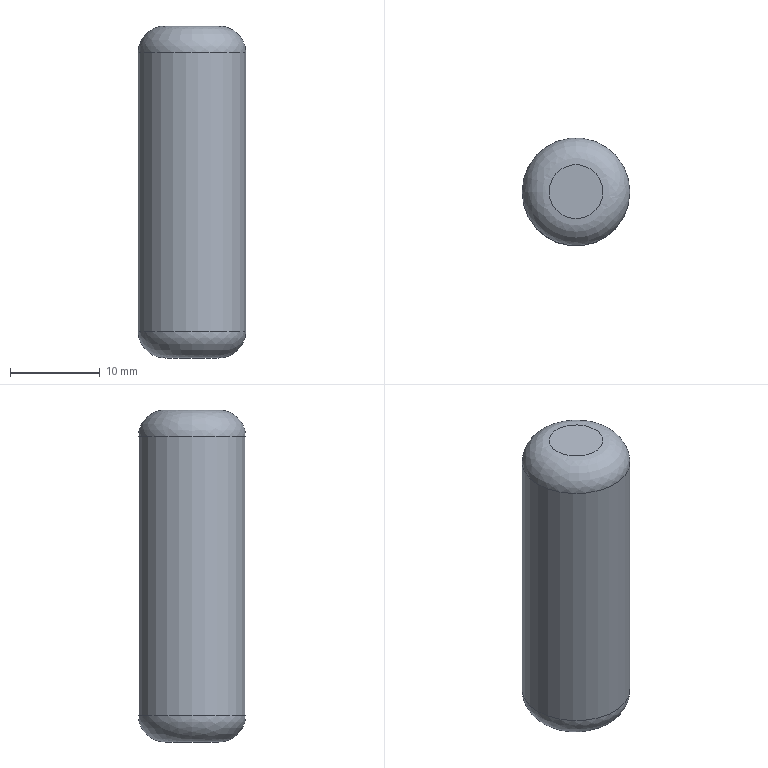Part | STEP file | Tube feed_id1566_x_t | 1 solid | 5 faces | box 12 x 12 x 37 mm | volume 4054 mm3 | plane 2 | spline 2 | cylinder 1 | commonest cylinder face diameters 12 x1
STEP:
#1=CARTESIAN_POINT('',(0.,0.,0.));
#2=DIRECTION('',(0.,0.,1.));
#3=DIRECTION('',(1.,0.,0.));
#4=AXIS2_PLACEMENT_3D('',#1,#2,#3);
#5=CARTESIAN_POINT('',(-15.,508.136,-235.));
#6=VERTEX_POINT('',#5);
#7=CARTESIAN_POINT('',(-9.,508.136,-235.));
#8=DIRECTION('',(0.,0.,1.));
#9=DIRECTION('',(-1.,0.,0.));
#10=AXIS2_PLACEMENT_3D('',#7,#8,#9);
#11=CIRCLE('',#10,6.);
#12=CARTESIAN_POINT('',(-9.,508.136,-201.));
#13=DIRECTION('',(0.,0.,-1.));
#14=DIRECTION('',(-1.,0.,0.));
#15=AXIS2_PLACEMENT_3D('',#12,#13,#14);
#16=CYLINDRICAL_SURFACE('',#15,6.);
#17=CARTESIAN_POINT('',(6.283,34.));
#18=DIRECTION('',(-1.,0.));
#19=VECTOR('',#18,1.);
#20=LINE('',#17,#19);
#21=(GEOMETRIC_REPRESENTATION_CONTEXT(2)PARAMETRIC_REPRESENTATION_CONTEXT()REPRESENTATION_CONTEXT('',''));
#22=DEFINITIONAL_REPRESENTATION('',(#20),#21);
#23=PCURVE('',#16,#22);
#24=CARTESIAN_POINT('',(-12.,508.136,-238.));
#25=CARTESIAN_POINT('',(-12.,514.136,-238.));
#26=CARTESIAN_POINT('',(-6.,514.136,-238.));
#27=CARTESIAN_POINT('',(-6.,508.136,-238.));
#28=CARTESIAN_POINT('',(-6.,502.136,-238.));
#29=CARTESIAN_POINT('',(-12.,502.136,-238.));
#30=CARTESIAN_POINT('',(-12.,508.136,-238.));
#31=CARTESIAN_POINT('',(-13.757,508.136,-238.));
#32=CARTESIAN_POINT('',(-13.757,517.65,-238.));
#33=CARTESIAN_POINT('',(-4.243,517.65,-238.));
#34=CARTESIAN_POINT('',(-4.243,508.136,-238.));
#35=CARTESIAN_POINT('',(-4.243,498.621,-238.));
#36=CARTESIAN_POINT('',(-13.757,498.621,-238.));
#37=CARTESIAN_POINT('',(-13.757,508.136,-238.));
#38=CARTESIAN_POINT('',(-15.,508.136,-236.757));
#39=CARTESIAN_POINT('',(-15.,520.136,-236.757));
#40=CARTESIAN_POINT('',(-3.,520.136,-236.757));
#41=CARTESIAN_POINT('',(-3.,508.136,-236.757));
#42=CARTESIAN_POINT('',(-3.,496.136,-236.757));
#43=CARTESIAN_POINT('',(-15.,496.136,-236.757));
#44=CARTESIAN_POINT('',(-15.,508.136,-236.757));
#45=CARTESIAN_POINT('',(-15.,508.136,-235.));
#46=CARTESIAN_POINT('',(-15.,520.136,-235.));
#47=CARTESIAN_POINT('',(-3.,520.136,-235.));
#48=CARTESIAN_POINT('',(-3.,508.136,-235.));
#49=CARTESIAN_POINT('',(-3.,496.136,-235.));
#50=CARTESIAN_POINT('',(-15.,496.136,-235.));
#51=CARTESIAN_POINT('',(-15.,508.136,-235.));
#52=(BOUNDED_SURFACE()B_SPLINE_SURFACE(3,3,((#24,#25,#26,#27,#28,#29,#30),(#31,#32,#33,#34,#35,#36,#37),(#38,#39,#40,#41,#42,#43,#44),(#45,#46,#47,#48,#49,#50,#51)),.UNSPECIFIED.,.F.,.T.,.F.)B_SPLINE_SURFACE_WITH_KNOTS((4,4),(1,3,3,3,1),(0.,1.),(-0.5,0.,0.5,1.,1.5),.UNSPECIFIED.)GEOMETRIC_REPRESENTATION_ITEM()RATIONAL_B_SPLINE_SURFACE(((1.,0.3333,0.3333,1.,0.3333,0.3333,1.),(0.8047,0.2682,0.2682,0.8047,0.2682,0.2682,0.8047),(0.8047,0.2682,0.2682,0.8047,0.2682,0.2682,0.8047),(1.,0.3333,0.3333,1.,0.3333,0.3333,1.)))REPRESENTATION_ITEM('')SURFACE());
#53=CARTESIAN_POINT('',(1.,1.));
#54=CARTESIAN_POINT('',(1.,0.9765));
#55=CARTESIAN_POINT('',(1.,0.9351));
#56=CARTESIAN_POINT('',(1.,0.8854));
#57=CARTESIAN_POINT('',(1.,0.8425));
#58=CARTESIAN_POINT('',(1.,0.804));
#59=CARTESIAN_POINT('',(1.,0.7678));
#60=CARTESIAN_POINT('',(1.,0.7322));
#61=CARTESIAN_POINT('',(1.,0.696));
#62=CARTESIAN_POINT('',(1.,0.6575));
#63=CARTESIAN_POINT('',(1.,0.6144));
#64=CARTESIAN_POINT('',(1.,0.5657));
#65=CARTESIAN_POINT('',(1.,0.5));
#66=CARTESIAN_POINT('',(1.,0.4343));
#67=CARTESIAN_POINT('',(1.,0.3856));
#68=CARTESIAN_POINT('',(1.,0.3425));
#69=CARTESIAN_POINT('',(1.,0.304));
#70=CARTESIAN_POINT('',(1.,0.2678));
#71=CARTESIAN_POINT('',(1.,0.2322));
#72=CARTESIAN_POINT('',(1.,0.196));
#73=CARTESIAN_POINT('',(1.,0.1575));
#74=CARTESIAN_POINT('',(1.,0.1146));
#75=CARTESIAN_POINT('',(1.,0.06491));
#76=CARTESIAN_POINT('',(1.,0.02352));
#77=CARTESIAN_POINT('',(1.,0.));
#78=B_SPLINE_CURVE_WITH_KNOTS('',3,(#53,#54,#55,#56,#57,#58,#59,#60,#61,#62,#63,#64,#65,#66,#67,#68,#69,#70,#71,#72,#73,#74,#75,#76,#77),.UNSPECIFIED.,.F.,.F.,(4,1,1,1,1,1,1,1,1,1,1,1,1,1,1,1,1,1,1,1,1,1,4),(0.,0.2856,0.5712,0.8568,1.142,1.428,1.714,1.999,2.285,2.57,2.856,3.142,3.427,3.713,3.998,4.284,4.57,4.855,5.141,5.426,5.712,5.998,6.283),.QUASI_UNIFORM_KNOTS.);
#79=(GEOMETRIC_REPRESENTATION_CONTEXT(2)PARAMETRIC_REPRESENTATION_CONTEXT()REPRESENTATION_CONTEXT('',''));
#80=DEFINITIONAL_REPRESENTATION('',(#78),#79);
#81=PCURVE('',#52,#80);
#82=SURFACE_CURVE('',#11,(#23,#81),.PCURVE_S1.);
#83=EDGE_CURVE('',#6,#6,#82,.T.);
#84=ORIENTED_EDGE('',*,*,#83,.T.);
#85=CARTESIAN_POINT('',(-15.,508.136,-204.));
#86=VERTEX_POINT('',#85);
#87=CARTESIAN_POINT('',(-15.,508.136,-204.));
#88=CARTESIAN_POINT('',(-15.,508.136,-235.));
#89=B_SPLINE_CURVE_WITH_KNOTS('',1,(#87,#88),.UNSPECIFIED.,.F.,.F.,(2,2),(3.,34.),.PIECEWISE_BEZIER_KNOTS.);
#90=CARTESIAN_POINT('',(0.,0.));
#91=DIRECTION('',(0.,1.));
#92=VECTOR('',#91,1.);
#93=LINE('',#90,#92);
#94=(GEOMETRIC_REPRESENTATION_CONTEXT(2)PARAMETRIC_REPRESENTATION_CONTEXT()REPRESENTATION_CONTEXT('',''));
#95=DEFINITIONAL_REPRESENTATION('',(#93),#94);
#96=PCURVE('',#16,#95);
#97=CARTESIAN_POINT('',(6.283,0.));
#98=DIRECTION('',(0.,1.));
#99=VECTOR('',#98,1.);
#100=LINE('',#97,#99);
#101=(GEOMETRIC_REPRESENTATION_CONTEXT(2)PARAMETRIC_REPRESENTATION_CONTEXT()REPRESENTATION_CONTEXT('',''));
#102=DEFINITIONAL_REPRESENTATION('',(#100),#101);
#103=PCURVE('',#16,#102);
#104=SEAM_CURVE('',#89,(#96,#103),.PCURVE_S1.);
#105=EDGE_CURVE('',#86,#6,#104,.T.);
#106=ORIENTED_EDGE('',*,*,#105,.F.);
#107=CARTESIAN_POINT('',(-9.,508.136,-204.));
#108=DIRECTION('',(0.,0.,-1.));
#109=DIRECTION('',(-1.,0.,0.));
#110=AXIS2_PLACEMENT_3D('',#107,#108,#109);
#111=CIRCLE('',#110,6.);
#112=CARTESIAN_POINT('',(0.,3.));
#113=DIRECTION('',(1.,0.));
#114=VECTOR('',#113,1.);
#115=LINE('',#112,#114);
#116=(GEOMETRIC_REPRESENTATION_CONTEXT(2)PARAMETRIC_REPRESENTATION_CONTEXT()REPRESENTATION_CONTEXT('',''));
#117=DEFINITIONAL_REPRESENTATION('',(#115),#116);
#118=PCURVE('',#16,#117);
#119=CARTESIAN_POINT('',(-15.,508.136,-204.));
#120=CARTESIAN_POINT('',(-15.,520.136,-204.));
#121=CARTESIAN_POINT('',(-3.,520.136,-204.));
#122=CARTESIAN_POINT('',(-3.,508.136,-204.));
#123=CARTESIAN_POINT('',(-3.,496.136,-204.));
#124=CARTESIAN_POINT('',(-15.,496.136,-204.));
#125=CARTESIAN_POINT('',(-15.,508.136,-204.));
#126=CARTESIAN_POINT('',(-15.,508.136,-202.243));
#127=CARTESIAN_POINT('',(-15.,520.136,-202.243));
#128=CARTESIAN_POINT('',(-3.,520.136,-202.243));
#129=CARTESIAN_POINT('',(-3.,508.136,-202.243));
#130=CARTESIAN_POINT('',(-3.,496.136,-202.243));
#131=CARTESIAN_POINT('',(-15.,496.136,-202.243));
#132=CARTESIAN_POINT('',(-15.,508.136,-202.243));
#133=CARTESIAN_POINT('',(-13.757,508.136,-201.));
#134=CARTESIAN_POINT('',(-13.757,517.65,-201.));
#135=CARTESIAN_POINT('',(-4.243,517.65,-201.));
#136=CARTESIAN_POINT('',(-4.243,508.136,-201.));
#137=CARTESIAN_POINT('',(-4.243,498.621,-201.));
#138=CARTESIAN_POINT('',(-13.757,498.621,-201.));
#139=CARTESIAN_POINT('',(-13.757,508.136,-201.));
#140=CARTESIAN_POINT('',(-12.,508.136,-201.));
#141=CARTESIAN_POINT('',(-12.,514.136,-201.));
#142=CARTESIAN_POINT('',(-6.,514.136,-201.));
#143=CARTESIAN_POINT('',(-6.,508.136,-201.));
#144=CARTESIAN_POINT('',(-6.,502.136,-201.));
#145=CARTESIAN_POINT('',(-12.,502.136,-201.));
#146=CARTESIAN_POINT('',(-12.,508.136,-201.));
#147=(BOUNDED_SURFACE()B_SPLINE_SURFACE(3,3,((#119,#120,#121,#122,#123,#124,#125),(#126,#127,#128,#129,#130,#131,#132),(#133,#134,#135,#136,#137,#138,#139),(#140,#141,#142,#143,#144,#145,#146)),.UNSPECIFIED.,.F.,.T.,.F.)B_SPLINE_SURFACE_WITH_KNOTS((4,4),(1,3,3,3,1),(0.,1.),(-0.5,0.,0.5,1.,1.5),.UNSPECIFIED.)GEOMETRIC_REPRESENTATION_ITEM()RATIONAL_B_SPLINE_SURFACE(((1.,0.3333,0.3333,1.,0.3333,0.3333,1.),(0.8047,0.2682,0.2682,0.8047,0.2682,0.2682,0.8047),(0.8047,0.2682,0.2682,0.8047,0.2682,0.2682,0.8047),(1.,0.3333,0.3333,1.,0.3333,0.3333,1.)))REPRESENTATION_ITEM('')SURFACE());
#148=CARTESIAN_POINT('',(0.,0.));
#149=CARTESIAN_POINT('',(0.,0.02352));
#150=CARTESIAN_POINT('',(0.,0.06491));
#151=CARTESIAN_POINT('',(0.,0.1146));
#152=CARTESIAN_POINT('',(0.,0.1575));
#153=CARTESIAN_POINT('',(0.,0.196));
#154=CARTESIAN_POINT('',(0.,0.2322));
#155=CARTESIAN_POINT('',(0.,0.2678));
#156=CARTESIAN_POINT('',(0.,0.304));
#157=CARTESIAN_POINT('',(0.,0.3425));
#158=CARTESIAN_POINT('',(0.,0.3856));
#159=CARTESIAN_POINT('',(0.,0.4343));
#160=CARTESIAN_POINT('',(0.,0.5));
#161=CARTESIAN_POINT('',(0.,0.5657));
#162=CARTESIAN_POINT('',(0.,0.6144));
#163=CARTESIAN_POINT('',(0.,0.6575));
#164=CARTESIAN_POINT('',(0.,0.696));
#165=CARTESIAN_POINT('',(0.,0.7322));
#166=CARTESIAN_POINT('',(0.,0.7678));
#167=CARTESIAN_POINT('',(0.,0.804));
#168=CARTESIAN_POINT('',(0.,0.8425));
#169=CARTESIAN_POINT('',(0.,0.8854));
#170=CARTESIAN_POINT('',(0.,0.9351));
#171=CARTESIAN_POINT('',(0.,0.9765));
#172=CARTESIAN_POINT('',(0.,1.));
#173=B_SPLINE_CURVE_WITH_KNOTS('',3,(#148,#149,#150,#151,#152,#153,#154,#155,#156,#157,#158,#159,#160,#161,#162,#163,#164,#165,#166,#167,#168,#169,#170,#171,#172),.UNSPECIFIED.,.F.,.F.,(4,1,1,1,1,1,1,1,1,1,1,1,1,1,1,1,1,1,1,1,1,1,4),(0.,0.2856,0.5712,0.8568,1.142,1.428,1.714,1.999,2.285,2.57,2.856,3.142,3.427,3.713,3.998,4.284,4.57,4.855,5.141,5.426,5.712,5.998,6.283),.QUASI_UNIFORM_KNOTS.);
#174=(GEOMETRIC_REPRESENTATION_CONTEXT(2)PARAMETRIC_REPRESENTATION_CONTEXT()REPRESENTATION_CONTEXT('',''));
#175=DEFINITIONAL_REPRESENTATION('',(#173),#174);
#176=PCURVE('',#147,#175);
#177=SURFACE_CURVE('',#111,(#118,#176),.PCURVE_S1.);
#178=EDGE_CURVE('',#86,#86,#177,.T.);
#179=ORIENTED_EDGE('',*,*,#178,.T.);
#180=ORIENTED_EDGE('',*,*,#105,.T.);
#181=EDGE_LOOP('',(#84,#106,#179,#180));
#182=FACE_BOUND('',#181,.T.);
#183=ADVANCED_FACE('',(#182),#16,.T.);
#184=CARTESIAN_POINT('',(-12.,508.136,-201.));
#185=VERTEX_POINT('',#184);
#186=CARTESIAN_POINT('',(-9.,508.136,-201.));
#187=DIRECTION('',(0.,0.,1.));
#188=DIRECTION('',(-1.,0.,0.));
#189=AXIS2_PLACEMENT_3D('',#186,#187,#188);
#190=CIRCLE('',#189,3.);
#191=CARTESIAN_POINT('',(-9.,508.136,-201.));
#192=DIRECTION('',(0.,0.,-1.));
#193=DIRECTION('',(-1.,0.,0.));
#194=AXIS2_PLACEMENT_3D('',#191,#192,#193);
#195=PLANE('',#194);
#196=CARTESIAN_POINT('',(3.,0.));
#197=CARTESIAN_POINT('',(3.,-5.196));
#198=CARTESIAN_POINT('',(-1.5,-2.598));
#199=CARTESIAN_POINT('',(-6.,0.));
#200=CARTESIAN_POINT('',(-1.5,2.598));
#201=CARTESIAN_POINT('',(3.,5.196));
#202=CARTESIAN_POINT('',(3.,0.));
#203=(BOUNDED_CURVE()B_SPLINE_CURVE(2,(#196,#197,#198,#199,#200,#201,#202),.UNSPECIFIED.,.T.,.F.)B_SPLINE_CURVE_WITH_KNOTS((1,2,2,2,2,1),(-2.094,0.,2.094,4.189,6.283,8.378),.UNSPECIFIED.)CURVE()GEOMETRIC_REPRESENTATION_ITEM()RATIONAL_B_SPLINE_CURVE((1.,0.5,1.,0.5,1.,0.5,1.))REPRESENTATION_ITEM(''));
#204=(GEOMETRIC_REPRESENTATION_CONTEXT(2)PARAMETRIC_REPRESENTATION_CONTEXT()REPRESENTATION_CONTEXT('',''));
#205=DEFINITIONAL_REPRESENTATION('',(#203),#204);
#206=PCURVE('',#195,#205);
#207=CARTESIAN_POINT('',(1.,1.));
#208=CARTESIAN_POINT('',(1.,0.9765));
#209=CARTESIAN_POINT('',(1.,0.9351));
#210=CARTESIAN_POINT('',(1.,0.8854));
#211=CARTESIAN_POINT('',(1.,0.8425));
#212=CARTESIAN_POINT('',(1.,0.804));
#213=CARTESIAN_POINT('',(1.,0.7678));
#214=CARTESIAN_POINT('',(1.,0.7322));
#215=CARTESIAN_POINT('',(1.,0.696));
#216=CARTESIAN_POINT('',(1.,0.6575));
#217=CARTESIAN_POINT('',(1.,0.6144));
#218=CARTESIAN_POINT('',(1.,0.5657));
#219=CARTESIAN_POINT('',(1.,0.5));
#220=CARTESIAN_POINT('',(1.,0.4343));
#221=CARTESIAN_POINT('',(1.,0.3856));
#222=CARTESIAN_POINT('',(1.,0.3425));
#223=CARTESIAN_POINT('',(1.,0.304));
#224=CARTESIAN_POINT('',(1.,0.2678));
#225=CARTESIAN_POINT('',(1.,0.2322));
#226=CARTESIAN_POINT('',(1.,0.196));
#227=CARTESIAN_POINT('',(1.,0.1575));
#228=CARTESIAN_POINT('',(1.,0.1146));
#229=CARTESIAN_POINT('',(1.,0.06491));
#230=CARTESIAN_POINT('',(1.,0.02352));
#231=CARTESIAN_POINT('',(1.,0.));
#232=B_SPLINE_CURVE_WITH_KNOTS('',3,(#207,#208,#209,#210,#211,#212,#213,#214,#215,#216,#217,#218,#219,#220,#221,#222,#223,#224,#225,#226,#227,#228,#229,#230,#231),.UNSPECIFIED.,.F.,.F.,(4,1,1,1,1,1,1,1,1,1,1,1,1,1,1,1,1,1,1,1,1,1,4),(0.,0.2856,0.5712,0.8568,1.142,1.428,1.714,1.999,2.285,2.57,2.856,3.142,3.427,3.713,3.998,4.284,4.57,4.855,5.141,5.426,5.712,5.998,6.283),.QUASI_UNIFORM_KNOTS.);
#233=(GEOMETRIC_REPRESENTATION_CONTEXT(2)PARAMETRIC_REPRESENTATION_CONTEXT()REPRESENTATION_CONTEXT('',''));
#234=DEFINITIONAL_REPRESENTATION('',(#232),#233);
#235=PCURVE('',#147,#234);
#236=SURFACE_CURVE('',#190,(#206,#235),.PCURVE_S1.);
#237=EDGE_CURVE('',#185,#185,#236,.T.);
#238=ORIENTED_EDGE('',*,*,#237,.T.);
#239=EDGE_LOOP('',(#238));
#240=FACE_BOUND('',#239,.T.);
#241=ADVANCED_FACE('',(#240),#195,.F.);
#242=CARTESIAN_POINT('',(-12.,508.136,-238.));
#243=VERTEX_POINT('',#242);
#244=CARTESIAN_POINT('',(-9.,508.136,-238.));
#245=DIRECTION('',(0.,0.,-1.));
#246=DIRECTION('',(-1.,0.,0.));
#247=AXIS2_PLACEMENT_3D('',#244,#245,#246);
#248=CIRCLE('',#247,3.);
#249=CARTESIAN_POINT('',(-9.,508.136,-238.));
#250=DIRECTION('',(0.,0.,-1.));
#251=DIRECTION('',(-1.,0.,0.));
#252=AXIS2_PLACEMENT_3D('',#249,#250,#251);
#253=PLANE('',#252);
#254=CARTESIAN_POINT('',(0.,0.));
#255=DIRECTION('',(1.,0.));
#256=AXIS2_PLACEMENT_2D('',#254,#255);
#257=CIRCLE('',#256,3.);
#258=(GEOMETRIC_REPRESENTATION_CONTEXT(2)PARAMETRIC_REPRESENTATION_CONTEXT()REPRESENTATION_CONTEXT('',''));
#259=DEFINITIONAL_REPRESENTATION('',(#257),#258);
#260=PCURVE('',#253,#259);
#261=CARTESIAN_POINT('',(0.,0.));
#262=CARTESIAN_POINT('',(0.,0.02352));
#263=CARTESIAN_POINT('',(0.,0.06491));
#264=CARTESIAN_POINT('',(0.,0.1146));
#265=CARTESIAN_POINT('',(0.,0.1575));
#266=CARTESIAN_POINT('',(0.,0.196));
#267=CARTESIAN_POINT('',(0.,0.2322));
#268=CARTESIAN_POINT('',(0.,0.2678));
#269=CARTESIAN_POINT('',(0.,0.304));
#270=CARTESIAN_POINT('',(0.,0.3425));
#271=CARTESIAN_POINT('',(0.,0.3856));
#272=CARTESIAN_POINT('',(0.,0.4343));
#273=CARTESIAN_POINT('',(0.,0.5));
#274=CARTESIAN_POINT('',(0.,0.5657));
#275=CARTESIAN_POINT('',(0.,0.6144));
#276=CARTESIAN_POINT('',(0.,0.6575));
#277=CARTESIAN_POINT('',(0.,0.696));
#278=CARTESIAN_POINT('',(0.,0.7322));
#279=CARTESIAN_POINT('',(0.,0.7678));
#280=CARTESIAN_POINT('',(0.,0.804));
#281=CARTESIAN_POINT('',(0.,0.8425));
#282=CARTESIAN_POINT('',(0.,0.8854));
#283=CARTESIAN_POINT('',(0.,0.9351));
#284=CARTESIAN_POINT('',(0.,0.9765));
#285=CARTESIAN_POINT('',(0.,1.));
#286=B_SPLINE_CURVE_WITH_KNOTS('',3,(#261,#262,#263,#264,#265,#266,#267,#268,#269,#270,#271,#272,#273,#274,#275,#276,#277,#278,#279,#280,#281,#282,#283,#284,#285),.UNSPECIFIED.,.F.,.F.,(4,1,1,1,1,1,1,1,1,1,1,1,1,1,1,1,1,1,1,1,1,1,4),(0.,0.2856,0.5712,0.8568,1.142,1.428,1.714,1.999,2.285,2.57,2.856,3.142,3.427,3.713,3.998,4.284,4.57,4.855,5.141,5.426,5.712,5.998,6.283),.QUASI_UNIFORM_KNOTS.);
#287=(GEOMETRIC_REPRESENTATION_CONTEXT(2)PARAMETRIC_REPRESENTATION_CONTEXT()REPRESENTATION_CONTEXT('',''));
#288=DEFINITIONAL_REPRESENTATION('',(#286),#287);
#289=PCURVE('',#52,#288);
#290=SURFACE_CURVE('',#248,(#260,#289),.PCURVE_S1.);
#291=EDGE_CURVE('',#243,#243,#290,.T.);
#292=ORIENTED_EDGE('',*,*,#291,.T.);
#293=EDGE_LOOP('',(#292));
#294=FACE_BOUND('',#293,.T.);
#295=ADVANCED_FACE('',(#294),#253,.T.);
#296=ORIENTED_EDGE('',*,*,#83,.F.);
#297=CARTESIAN_POINT('',(-12.,508.136,-238.));
#298=CARTESIAN_POINT('',(-13.757,508.136,-238.));
#299=CARTESIAN_POINT('',(-15.,508.136,-236.757));
#300=CARTESIAN_POINT('',(-15.,508.136,-235.));
#301=(BOUNDED_CURVE()B_SPLINE_CURVE(3,(#297,#298,#299,#300),.UNSPECIFIED.,.F.,.F.)B_SPLINE_CURVE_WITH_KNOTS((4,4),(0.,1.),.PIECEWISE_BEZIER_KNOTS.)CURVE()GEOMETRIC_REPRESENTATION_ITEM()RATIONAL_B_SPLINE_CURVE((1.,0.8047,0.8047,1.))REPRESENTATION_ITEM(''));
#302=CARTESIAN_POINT('',(0.,1.));
#303=DIRECTION('',(1.,0.));
#304=VECTOR('',#303,1.);
#305=LINE('',#302,#304);
#306=(GEOMETRIC_REPRESENTATION_CONTEXT(2)PARAMETRIC_REPRESENTATION_CONTEXT()REPRESENTATION_CONTEXT('',''));
#307=DEFINITIONAL_REPRESENTATION('',(#305),#306);
#308=PCURVE('',#52,#307);
#309=CARTESIAN_POINT('',(0.,0.));
#310=DIRECTION('',(1.,0.));
#311=VECTOR('',#310,1.);
#312=LINE('',#309,#311);
#313=(GEOMETRIC_REPRESENTATION_CONTEXT(2)PARAMETRIC_REPRESENTATION_CONTEXT()REPRESENTATION_CONTEXT('',''));
#314=DEFINITIONAL_REPRESENTATION('',(#312),#313);
#315=PCURVE('',#52,#314);
#316=SEAM_CURVE('',#301,(#308,#315),.PCURVE_S1.);
#317=EDGE_CURVE('',#243,#6,#316,.T.);
#318=ORIENTED_EDGE('',*,*,#317,.F.);
#319=ORIENTED_EDGE('',*,*,#291,.F.);
#320=ORIENTED_EDGE('',*,*,#317,.T.);
#321=EDGE_LOOP('',(#296,#318,#319,#320));
#322=FACE_BOUND('',#321,.T.);
#323=ADVANCED_FACE('',(#322),#52,.T.);
#324=ORIENTED_EDGE('',*,*,#237,.F.);
#325=CARTESIAN_POINT('',(-15.,508.136,-204.));
#326=CARTESIAN_POINT('',(-15.,508.136,-202.243));
#327=CARTESIAN_POINT('',(-13.757,508.136,-201.));
#328=CARTESIAN_POINT('',(-12.,508.136,-201.));
#329=(BOUNDED_CURVE()B_SPLINE_CURVE(3,(#325,#326,#327,#328),.UNSPECIFIED.,.F.,.F.)B_SPLINE_CURVE_WITH_KNOTS((4,4),(0.,1.),.PIECEWISE_BEZIER_KNOTS.)CURVE()GEOMETRIC_REPRESENTATION_ITEM()RATIONAL_B_SPLINE_CURVE((1.,0.8047,0.8047,1.))REPRESENTATION_ITEM(''));
#330=CARTESIAN_POINT('',(0.,1.));
#331=DIRECTION('',(1.,0.));
#332=VECTOR('',#331,1.);
#333=LINE('',#330,#332);
#334=(GEOMETRIC_REPRESENTATION_CONTEXT(2)PARAMETRIC_REPRESENTATION_CONTEXT()REPRESENTATION_CONTEXT('',''));
#335=DEFINITIONAL_REPRESENTATION('',(#333),#334);
#336=PCURVE('',#147,#335);
#337=CARTESIAN_POINT('',(0.,0.));
#338=DIRECTION('',(1.,0.));
#339=VECTOR('',#338,1.);
#340=LINE('',#337,#339);
#341=(GEOMETRIC_REPRESENTATION_CONTEXT(2)PARAMETRIC_REPRESENTATION_CONTEXT()REPRESENTATION_CONTEXT('',''));
#342=DEFINITIONAL_REPRESENTATION('',(#340),#341);
#343=PCURVE('',#147,#342);
#344=SEAM_CURVE('',#329,(#336,#343),.PCURVE_S1.);
#345=EDGE_CURVE('',#86,#185,#344,.T.);
#346=ORIENTED_EDGE('',*,*,#345,.F.);
#347=ORIENTED_EDGE('',*,*,#178,.F.);
#348=ORIENTED_EDGE('',*,*,#345,.T.);
#349=EDGE_LOOP('',(#324,#346,#347,#348));
#350=FACE_BOUND('',#349,.T.);
#351=ADVANCED_FACE('',(#350),#147,.T.);
#352=CLOSED_SHELL('',(#183,#241,#295,#323,#351));
#353=MANIFOLD_SOLID_BREP('',#352);
#354=(LENGTH_UNIT()NAMED_UNIT(*)SI_UNIT(.MILLI.,.METRE.));
#355=UNCERTAINTY_MEASURE_WITH_UNIT(LENGTH_MEASURE(0.00001),#354,'','');
#356=(NAMED_UNIT(*)PLANE_ANGLE_UNIT()SI_UNIT($,.RADIAN.));
#357=(NAMED_UNIT(*)SI_UNIT($,.STERADIAN.)SOLID_ANGLE_UNIT());
#358=(GEOMETRIC_REPRESENTATION_CONTEXT(3)GLOBAL_UNCERTAINTY_ASSIGNED_CONTEXT((#355))GLOBAL_UNIT_ASSIGNED_CONTEXT((#354,#356,#357))REPRESENTATION_CONTEXT('',''));
#359=ADVANCED_BREP_SHAPE_REPRESENTATION('',(#4,#353),#358);